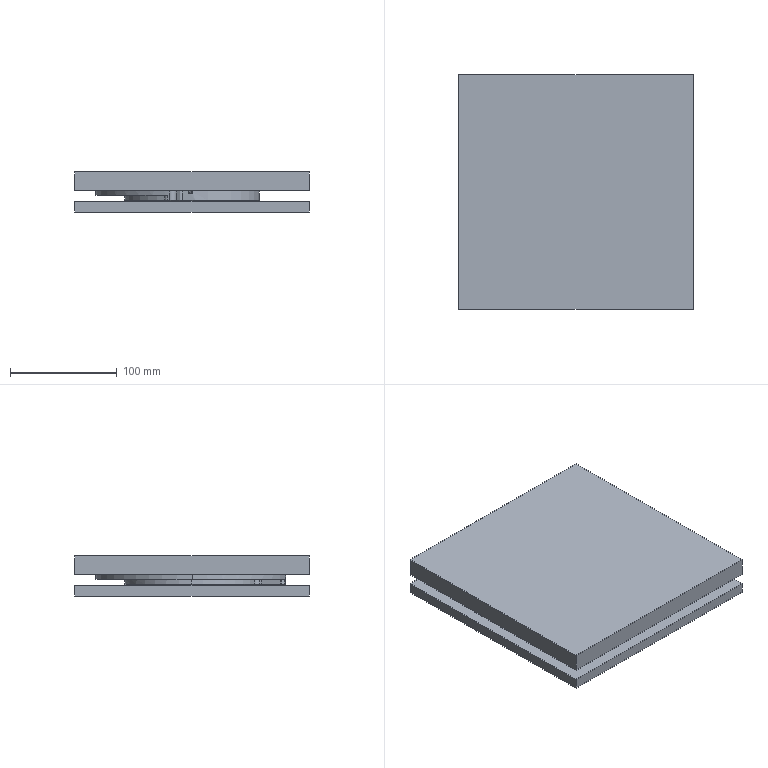NC program | NX | posted with a generic post | part box 220 x 220 x 37.5 mm
Lines 3644 to 4913 of 13716:
(ZLEVEL_PROFILE_COPY , TOOL : D10JING)
N7250 T07 M6
N7252 G54
N7254 G17 G0 G90 X87.471 Y-41.927 S8000 M3
N7256 G43 Z30. H7
N7258 Z-17.
N7260 G94 G1 X85.759 Y-42.028 F1200.
N7262 G3 X84.924 Y-42.578 R1.
N7264 G2 X70.985 Y-46.757 R10.
N7266 G1 X56.243 Y-38.246
N7268 X56.225 Y-38.248
N7270 X55.355 Y-39.494
N7272 G2 X55.057 Y-39.91 R68.
N7274 G1 X54.666 Y-40.443
N7276 G2 X52.455 Y-43.272 R68.
N7278 G1 X52.409 Y-43.328
N7280 G2 X-67.991 Y-1.079 R68.
N7282 G1 X-67.995 Y0.834
N7284 G2 X-67.897 Y3.74 R68.
N7286 G1 X-67.853 Y4.42
N7288 X-67.856 Y4.43
N7290 G2 X-67.657 Y6.818 R68.
N7292 G1 X-67.652 Y6.852
N7294 X-84.432 Y9.81
N7296 G2 X-92.427 Y21.958 R10.
N7298 G1 X-92.42 Y21.99
N7300 G3 X-92.706 Y22.949 R1.
N7302 G1 X-93.952 Y24.125
N7304 G0 Z30.
N7306 M5
(ZLEVEL_PROFILE_COPY_1 , TOOL : D6)
N7308 T09 M6
N7310 G54
N7312 G17 G0 G90 X38.681 Y9.135 S9500 M3
N7314 G43 Z30. H9
N7316 Z-0.5
N7318 G94 G1 X37.71 Y9.242 F1000.
N7320 G3 X37.511 Y8.676 R0.6
N7322 G1 X37.527 Y8.601 F1500.
N7324 G2 X37.907 Y6.73 R38.5
N7326 G1 X39.921 Y6.928
N7328 G3 X40.409 Y7.277 R0.6
N7330 G1 X40.838 Y8.223
N7332 G0 X38.681 Y9.135 Z-1.
N7334 G1 X37.71 Y9.242 F1000.
N7336 G3 X37.511 Y8.676 R0.6
N7338 G1 X37.527 Y8.601 F1500.
N7340 G2 X37.907 Y6.73 R38.5
N7342 G1 X39.921 Y6.928
N7344 G3 X40.409 Y7.277 R0.6
N7346 G1 X40.838 Y8.223
N7348 G0 X38.681 Y9.135 Z-1.5
N7350 G1 X37.71 Y9.242 F1000.
N7352 G3 X37.511 Y8.676 R0.6
N7354 G1 X37.527 Y8.601 F1500.
N7356 G2 X37.907 Y6.73 R38.5
N7358 G1 X39.921 Y6.928
N7360 G3 X40.409 Y7.277 R0.6
N7362 G1 X40.838 Y8.223
N7364 G0 X38.681 Y9.135 Z-2.
N7366 G1 X37.71 Y9.242 F1000.
N7368 G3 X37.511 Y8.676 R0.6
N7370 G1 X37.527 Y8.601 F1500.
N7372 G2 X37.907 Y6.73 R38.5
N7374 G1 X39.921 Y6.928
N7376 G3 X40.409 Y7.277 R0.6
N7378 G1 X40.838 Y8.223
N7380 G0 X38.681 Y9.135 Z-2.5
N7382 G1 X37.71 Y9.242 F1000.
N7384 G3 X37.511 Y8.676 R0.6
N7386 G1 X37.527 Y8.601 F1500.
N7388 G2 X37.907 Y6.73 R38.5
N7390 G1 X39.921 Y6.928
N7392 G3 X40.409 Y7.277 R0.6
N7394 G1 X40.838 Y8.223
N7396 G0 X38.681 Y9.135 Z-3.
N7398 G1 X37.71 Y9.242 F1000.
N7400 G3 X37.511 Y8.676 R0.6
N7402 G1 X37.527 Y8.601 F1500.
N7404 G2 X37.907 Y6.73 R38.5
N7406 G1 X39.921 Y6.928
N7408 G3 X40.409 Y7.277 R0.6
N7410 G1 X40.838 Y8.223
N7412 G0 X38.681 Y9.135 Z-3.5
N7414 G1 X37.71 Y9.242 F1000.
N7416 G3 X37.511 Y8.676 R0.6
N7418 G1 X37.527 Y8.601 F1500.
N7420 G2 X37.907 Y6.73 R38.5
N7422 G1 X39.921 Y6.928
N7424 G3 X40.409 Y7.277 R0.6
N7426 G1 X40.838 Y8.223
N7428 G0 X38.681 Y9.135 Z-4.
N7430 G1 X37.71 Y9.242 F1000.
N7432 G3 X37.511 Y8.676 R0.6
N7434 G1 X37.527 Y8.601 F1500.
N7436 G2 X37.907 Y6.73 R38.5
N7438 G1 X39.921 Y6.928
N7440 G3 X40.409 Y7.277 R0.6
N7442 G1 X40.838 Y8.223
N7444 G0 X38.681 Y9.135 Z-4.5
N7446 G1 X37.71 Y9.242 F1000.
N7448 G3 X37.511 Y8.676 R0.6
N7450 G1 X37.527 Y8.601 F1500.
N7452 G2 X37.907 Y6.73 R38.5
N7454 G1 X39.921 Y6.928
N7456 G3 X40.409 Y7.277 R0.6
N7458 G1 X40.838 Y8.223
N7460 G0 X38.681 Y9.135 Z-5.
N7462 G1 X37.71 Y9.242 F1000.
N7464 G3 X37.511 Y8.676 R0.6
N7466 G1 X37.527 Y8.601 F1500.
N7468 G2 X37.907 Y6.73 R38.5
N7470 G1 X39.921 Y6.928
N7472 G3 X40.409 Y7.277 R0.6
N7474 G1 X40.838 Y8.223
N7476 G0 X38.681 Y9.135 Z-5.5
N7478 G1 X37.71 Y9.242 F1000.
N7480 G3 X37.511 Y8.676 R0.6
N7482 G1 X37.527 Y8.601 F1500.
N7484 G2 X37.907 Y6.73 R38.5
N7486 G1 X39.921 Y6.928
N7488 G3 X40.409 Y7.277 R0.6
N7490 G1 X40.838 Y8.223
N7492 G0 X38.681 Y9.135 Z-6.
N7494 G1 X37.71 Y9.242 F1000.
N7496 G3 X37.511 Y8.676 R0.6
N7498 G1 X37.527 Y8.601 F1500.
N7500 G2 X37.907 Y6.73 R38.5
N7502 G1 X39.921 Y6.928
N7504 G3 X40.409 Y7.277 R0.6
N7506 G1 X40.838 Y8.223
N7508 G0 X38.681 Y9.135 Z-6.5
N7510 G1 X37.71 Y9.242 F1000.
N7512 G3 X37.511 Y8.676 R0.6
N7514 G1 X37.527 Y8.601 F1500.
N7516 G2 X37.907 Y6.73 R38.5
N7518 G1 X39.921 Y6.928
N7520 G3 X40.409 Y7.277 R0.6
N7522 G1 X40.838 Y8.223
N7524 G0 X38.681 Y9.135 Z-7.
N7526 G1 X37.71 Y9.242 F1000.
N7528 G3 X37.511 Y8.676 R0.6
N7530 G1 X37.527 Y8.601 F1500.
N7532 G2 X37.907 Y6.73 R38.5
N7534 G1 X39.921 Y6.928
N7536 G3 X40.409 Y7.277 R0.6
N7538 G1 X40.838 Y8.223
N7540 G0 X38.681 Y9.135 Z-7.5
N7542 G1 X37.71 Y9.242 F1000.
N7544 G3 X37.511 Y8.676 R0.6
N7546 G1 X37.527 Y8.601 F1500.
N7548 G2 X37.907 Y6.73 R38.5
N7550 G1 X39.921 Y6.928
N7552 G3 X40.409 Y7.277 R0.6
N7554 G1 X40.838 Y8.223
N7556 G0 X38.681 Y9.135 Z-8.
N7558 G1 X37.71 Y9.242 F1000.
N7560 G3 X37.511 Y8.676 R0.6
N7562 G1 X37.527 Y8.601 F1500.
N7564 G2 X37.907 Y6.73 R38.5
N7566 G1 X39.921 Y6.928
N7568 G3 X40.409 Y7.277 R0.6
N7570 G1 X40.838 Y8.223
N7572 G0 X38.681 Y9.135 Z-8.5
N7574 G1 X37.71 Y9.242 F1000.
N7576 G3 X37.511 Y8.676 R0.6
N7578 G1 X37.527 Y8.601 F1500.
N7580 G2 X37.907 Y6.73 R38.5
N7582 G1 X39.921 Y6.928
N7584 G3 X40.409 Y7.277 R0.6
N7586 G1 X40.838 Y8.223
N7588 G0 X38.681 Y9.135 Z-9.
N7590 G1 X37.71 Y9.242 F1000.
N7592 G3 X37.511 Y8.676 R0.6
N7594 G1 X37.527 Y8.601 F1500.
N7596 G2 X37.907 Y6.73 R38.5
N7598 G1 X39.921 Y6.928
N7600 G3 X40.409 Y7.277 R0.6
N7602 G1 X40.838 Y8.223
N7604 G0 X38.681 Y9.135 Z-9.5
N7606 G1 X37.71 Y9.242 F1000.
N7608 G3 X37.511 Y8.676 R0.6
N7610 G1 X37.527 Y8.601 F1500.
N7612 G2 X37.907 Y6.73 R38.5
N7614 G1 X39.921 Y6.928
N7616 G3 X40.409 Y7.277 R0.6
N7618 G1 X40.838 Y8.223
N7620 G0 X38.681 Y9.135 Z-10.
N7622 G1 X37.71 Y9.242 F1000.
N7624 G3 X37.511 Y8.676 R0.6
N7626 G1 X37.527 Y8.601 F1500.
N7628 G2 X37.907 Y6.73 R38.5
N7630 G1 X39.921 Y6.928
N7632 G3 X40.409 Y7.277 R0.6
N7634 G1 X40.838 Y8.223
N7636 G0 Z30.
N7638 X39.099 Y-14.376
N7640 Z-0.5
N7642 G1 X38.819 Y-13.375 F1000.
N7644 G3 X38.391 Y-12.955 R0.6
N7646 G1 X36.431 Y-12.452 F1500.
N7648 G2 X35.74 Y-14.314 R38.5
N7650 G3 X35.826 Y-14.908 R0.6
N7652 G1 X36.458 Y-15.712
N7654 G0 X39.099 Y-14.376 Z-1.
N7656 G1 X38.819 Y-13.375 F1000.
N7658 G3 X38.391 Y-12.955 R0.6
N7660 G1 X36.431 Y-12.452 F1500.
N7662 G2 X35.74 Y-14.314 R38.5
N7664 G3 X35.826 Y-14.908 R0.6
N7666 G1 X36.458 Y-15.712
N7668 G0 X39.099 Y-14.376 Z-1.5
N7670 G1 X38.819 Y-13.375 F1000.
N7672 G3 X38.391 Y-12.955 R0.6
N7674 G1 X36.431 Y-12.452 F1500.
N7676 G2 X35.74 Y-14.314 R38.5
N7678 G3 X35.826 Y-14.908 R0.6
N7680 G1 X36.458 Y-15.712
N7682 G0 X39.099 Y-14.376 Z-2.
N7684 G1 X38.819 Y-13.375 F1000.
N7686 G3 X38.391 Y-12.955 R0.6
N7688 G1 X36.431 Y-12.452 F1500.
N7690 G2 X35.74 Y-14.314 R38.5
N7692 G3 X35.826 Y-14.908 R0.6
N7694 G1 X36.458 Y-15.712
N7696 G0 X39.099 Y-14.376 Z-2.5
N7698 G1 X38.819 Y-13.375 F1000.
N7700 G3 X38.391 Y-12.955 R0.6
N7702 G1 X36.431 Y-12.452 F1500.
N7704 G2 X35.74 Y-14.314 R38.5
N7706 G3 X35.826 Y-14.908 R0.6
N7708 G1 X36.458 Y-15.712
N7710 G0 X39.099 Y-14.376 Z-3.
N7712 G1 X38.819 Y-13.375 F1000.
N7714 G3 X38.391 Y-12.955 R0.6
N7716 G1 X36.431 Y-12.452 F1500.
N7718 G2 X35.74 Y-14.314 R38.5
N7720 G3 X35.826 Y-14.908 R0.6
N7722 G1 X36.458 Y-15.712
N7724 G0 X39.099 Y-14.376 Z-3.5
N7726 G1 X38.819 Y-13.375 F1000.
N7728 G3 X38.391 Y-12.955 R0.6
N7730 G1 X36.431 Y-12.452 F1500.
N7732 G2 X35.74 Y-14.314 R38.5
N7734 G3 X35.826 Y-14.908 R0.6
N7736 G1 X36.458 Y-15.712
N7738 G0 X39.099 Y-14.376 Z-4.
N7740 G1 X38.819 Y-13.375 F1000.
N7742 G3 X38.391 Y-12.955 R0.6
N7744 G1 X36.431 Y-12.452 F1500.
N7746 G2 X35.74 Y-14.314 R38.5
N7748 G3 X35.826 Y-14.908 R0.6
N7750 G1 X36.458 Y-15.712
N7752 G0 X39.099 Y-14.376 Z-4.5
N7754 G1 X38.819 Y-13.375 F1000.
N7756 G3 X38.391 Y-12.955 R0.6
N7758 G1 X36.431 Y-12.452 F1500.
N7760 G2 X35.74 Y-14.314 R38.5
N7762 G3 X35.826 Y-14.908 R0.6
N7764 G1 X36.458 Y-15.712
N7766 G0 X39.099 Y-14.376 Z-5.
N7768 G1 X38.819 Y-13.375 F1000.
N7770 G3 X38.391 Y-12.955 R0.6
N7772 G1 X36.431 Y-12.452 F1500.
N7774 G2 X35.74 Y-14.314 R38.5
N7776 G3 X35.826 Y-14.908 R0.6
N7778 G1 X36.458 Y-15.712
N7780 G0 X39.099 Y-14.376 Z-5.5
N7782 G1 X38.819 Y-13.375 F1000.
N7784 G3 X38.391 Y-12.955 R0.6
N7786 G1 X36.431 Y-12.452 F1500.
N7788 G2 X35.74 Y-14.314 R38.5
N7790 G3 X35.826 Y-14.908 R0.6
N7792 G1 X36.458 Y-15.712
N7794 G0 X39.099 Y-14.376 Z-6.
N7796 G1 X38.819 Y-13.375 F1000.
N7798 G3 X38.391 Y-12.955 R0.6
N7800 G1 X36.431 Y-12.452 F1500.
N7802 G2 X35.74 Y-14.314 R38.5
N7804 G3 X35.826 Y-14.908 R0.6
N7806 G1 X36.458 Y-15.712
N7808 G0 X39.099 Y-14.376 Z-6.5
N7810 G1 X38.819 Y-13.375 F1000.
N7812 G3 X38.391 Y-12.955 R0.6
N7814 G1 X36.431 Y-12.452 F1500.
N7816 G2 X35.74 Y-14.314 R38.5
N7818 G3 X35.826 Y-14.908 R0.6
N7820 G1 X36.458 Y-15.712
N7822 G0 X39.099 Y-14.376 Z-7.
N7824 G1 X38.819 Y-13.375 F1000.
N7826 G3 X38.391 Y-12.955 R0.6
N7828 G1 X36.431 Y-12.452 F1500.
N7830 G2 X35.74 Y-14.314 R38.5
N7832 G3 X35.826 Y-14.908 R0.6
N7834 G1 X36.458 Y-15.712
N7836 G0 X39.099 Y-14.376 Z-7.5
N7838 G1 X38.819 Y-13.375 F1000.
N7840 G3 X38.391 Y-12.955 R0.6
N7842 G1 X36.431 Y-12.452 F1500.
N7844 G2 X35.74 Y-14.314 R38.5
N7846 G3 X35.826 Y-14.908 R0.6
N7848 G1 X36.458 Y-15.712
N7850 G0 X39.099 Y-14.376 Z-8.
N7852 G1 X38.819 Y-13.375 F1000.
N7854 G3 X38.391 Y-12.955 R0.6
N7856 G1 X36.431 Y-12.452 F1500.
N7858 G2 X35.74 Y-14.314 R38.5
N7860 G3 X35.826 Y-14.908 R0.6
N7862 G1 X36.458 Y-15.712
N7864 G0 X39.099 Y-14.376 Z-8.5
N7866 G1 X38.819 Y-13.375 F1000.
N7868 G3 X38.391 Y-12.955 R0.6
N7870 G1 X36.431 Y-12.452 F1500.
N7872 G2 X35.74 Y-14.314 R38.5
N7874 G3 X35.826 Y-14.908 R0.6
N7876 G1 X36.458 Y-15.712
N7878 G0 X39.099 Y-14.376 Z-9.
N7880 G1 X38.819 Y-13.375 F1000.
N7882 G3 X38.391 Y-12.955 R0.6
N7884 G1 X36.431 Y-12.452 F1500.
N7886 G2 X35.74 Y-14.314 R38.5
N7888 G3 X35.826 Y-14.908 R0.6
N7890 G1 X36.458 Y-15.712
N7892 G0 X39.099 Y-14.376 Z-9.5
N7894 G1 X38.819 Y-13.375 F1000.
N7896 G3 X38.391 Y-12.955 R0.6
N7898 G1 X36.431 Y-12.452 F1500.
N7900 G2 X35.74 Y-14.314 R38.5
N7902 G3 X35.826 Y-14.908 R0.6
N7904 G1 X36.458 Y-15.712
N7906 G0 X39.099 Y-14.376 Z-10.
N7908 G1 X38.819 Y-13.375 F1000.
N7910 G3 X38.391 Y-12.955 R0.6
N7912 G1 X36.431 Y-12.452 F1500.
N7914 G2 X35.74 Y-14.314 R38.5
N7916 G3 X35.826 Y-14.908 R0.6
N7918 G1 X36.458 Y-15.712
N7920 G0 Z30.
N7922 X-33.176 Y-21.805
N7924 Z-0.5
N7926 G1 X-32.693 Y-20.902 F1000.
N7928 G3 X-32.712 Y-20.302 R0.6
N7930 G2 X-33.715 Y-18.589 R38.5 F1500.
N7932 G1 X-35.558 Y-19.425
N7934 G3 X-35.907 Y-19.913 R0.6
N7936 G1 X-36.009 Y-20.947
N7938 G0 X-33.176 Y-21.805 Z-1.
N7940 G1 X-32.693 Y-20.902 F1000.
N7942 G3 X-32.712 Y-20.302 R0.6
N7944 G2 X-33.715 Y-18.589 R38.5 F1500.
N7946 G1 X-35.558 Y-19.425
N7948 G3 X-35.907 Y-19.913 R0.6
N7950 G1 X-36.009 Y-20.947
N7952 G0 X-33.176 Y-21.805 Z-1.5
N7954 G1 X-32.693 Y-20.902 F1000.
N7956 G3 X-32.712 Y-20.302 R0.6
N7958 G2 X-33.715 Y-18.589 R38.5 F1500.
N7960 G1 X-35.558 Y-19.425
N7962 G3 X-35.907 Y-19.913 R0.6
N7964 G1 X-36.009 Y-20.947
N7966 G0 X-33.176 Y-21.805 Z-2.
N7968 G1 X-32.693 Y-20.902 F1000.
N7970 G3 X-32.712 Y-20.302 R0.6
N7972 G2 X-33.715 Y-18.589 R38.5 F1500.
N7974 G1 X-35.558 Y-19.425
N7976 G3 X-35.907 Y-19.913 R0.6
N7978 G1 X-36.009 Y-20.947
N7980 G0 X-33.176 Y-21.805 Z-2.5
N7982 G1 X-32.693 Y-20.902 F1000.
N7984 G3 X-32.712 Y-20.302 R0.6
N7986 G2 X-33.715 Y-18.589 R38.5 F1500.
N7988 G1 X-35.558 Y-19.425
N7990 G3 X-35.907 Y-19.913 R0.6
N7992 G1 X-36.009 Y-20.947
N7994 G0 X-33.176 Y-21.805 Z-3.
N7996 G1 X-32.693 Y-20.902 F1000.
N7998 G3 X-32.712 Y-20.302 R0.6
N8000 G2 X-33.715 Y-18.589 R38.5 F1500.
N8002 G1 X-35.558 Y-19.425
N8004 G3 X-35.907 Y-19.913 R0.6
N8006 G1 X-36.009 Y-20.947
N8008 G0 X-33.176 Y-21.805 Z-3.5
N8010 G1 X-32.693 Y-20.902 F1000.
N8012 G3 X-32.712 Y-20.302 R0.6
N8014 G2 X-33.715 Y-18.589 R38.5 F1500.
N8016 G1 X-35.558 Y-19.425
N8018 G3 X-35.907 Y-19.913 R0.6
N8020 G1 X-36.009 Y-20.947
N8022 G0 X-33.176 Y-21.805 Z-4.
N8024 G1 X-32.693 Y-20.902 F1000.
N8026 G3 X-32.712 Y-20.302 R0.6
N8028 G2 X-33.715 Y-18.589 R38.5 F1500.
N8030 G1 X-35.558 Y-19.425
N8032 G3 X-35.907 Y-19.913 R0.6
N8034 G1 X-36.009 Y-20.947
N8036 G0 X-33.176 Y-21.805 Z-4.5
N8038 G1 X-32.693 Y-20.902 F1000.
N8040 G3 X-32.712 Y-20.302 R0.6
N8042 G2 X-33.715 Y-18.589 R38.5 F1500.
N8044 G1 X-35.558 Y-19.425
N8046 G3 X-35.907 Y-19.913 R0.6
N8048 G1 X-36.009 Y-20.947
N8050 G0 X-33.176 Y-21.805 Z-5.
N8052 G1 X-32.693 Y-20.902 F1000.
N8054 G3 X-32.712 Y-20.302 R0.6
N8056 G2 X-33.715 Y-18.589 R38.5 F1500.
N8058 G1 X-35.558 Y-19.425
N8060 G3 X-35.907 Y-19.913 R0.6
N8062 G1 X-36.009 Y-20.947
N8064 G0 X-33.176 Y-21.805 Z-5.5
N8066 G1 X-32.693 Y-20.902 F1000.
N8068 G3 X-32.712 Y-20.302 R0.6
N8070 G2 X-33.715 Y-18.589 R38.5 F1500.
N8072 G1 X-35.558 Y-19.425
N8074 G3 X-35.907 Y-19.913 R0.6
N8076 G1 X-36.009 Y-20.947
N8078 G0 X-33.176 Y-21.805 Z-6.
N8080 G1 X-32.693 Y-20.902 F1000.
N8082 G3 X-32.712 Y-20.302 R0.6
N8084 G2 X-33.715 Y-18.589 R38.5 F1500.
N8086 G1 X-35.558 Y-19.425
N8088 G3 X-35.907 Y-19.913 R0.6
N8090 G1 X-36.009 Y-20.947
N8092 G0 X-33.176 Y-21.805 Z-6.5
N8094 G1 X-32.693 Y-20.902 F1000.
N8096 G3 X-32.712 Y-20.302 R0.6
N8098 G2 X-33.715 Y-18.589 R38.5 F1500.
N8100 G1 X-35.558 Y-19.425
N8102 G3 X-35.907 Y-19.913 R0.6
N8104 G1 X-36.009 Y-20.947
N8106 G0 X-33.176 Y-21.805 Z-7.
N8108 G1 X-32.693 Y-20.902 F1000.
N8110 G3 X-32.712 Y-20.302 R0.6
N8112 G2 X-33.715 Y-18.589 R38.5 F1500.
N8114 G1 X-35.558 Y-19.425
N8116 G3 X-35.907 Y-19.913 R0.6
N8118 G1 X-36.009 Y-20.947
N8120 G0 X-33.176 Y-21.805 Z-7.5
N8122 G1 X-32.693 Y-20.902 F1000.
N8124 G3 X-32.712 Y-20.302 R0.6
N8126 G2 X-33.715 Y-18.589 R38.5 F1500.
N8128 G1 X-35.558 Y-19.425
N8130 G3 X-35.907 Y-19.913 R0.6
N8132 G1 X-36.009 Y-20.947
N8134 G0 X-33.176 Y-21.805 Z-8.
N8136 G1 X-32.693 Y-20.902 F1000.
N8138 G3 X-32.712 Y-20.302 R0.6
N8140 G2 X-33.715 Y-18.589 R38.5 F1500.
N8142 G1 X-35.558 Y-19.425
N8144 G3 X-35.907 Y-19.913 R0.6
N8146 G1 X-36.009 Y-20.947
N8148 G0 X-33.176 Y-21.805 Z-8.5
N8150 G1 X-32.693 Y-20.902 F1000.
N8152 G3 X-32.712 Y-20.302 R0.6
N8154 G2 X-33.715 Y-18.589 R38.5 F1500.
N8156 G1 X-35.558 Y-19.425
N8158 G3 X-35.907 Y-19.913 R0.6
N8160 G1 X-36.009 Y-20.947
N8162 G0 X-33.176 Y-21.805 Z-9.
N8164 G1 X-32.693 Y-20.902 F1000.
N8166 G3 X-32.712 Y-20.302 R0.6
N8168 G2 X-33.715 Y-18.589 R38.5 F1500.
N8170 G1 X-35.558 Y-19.425
N8172 G3 X-35.907 Y-19.913 R0.6
N8174 G1 X-36.009 Y-20.947
N8176 G0 X-33.176 Y-21.805 Z-9.5
N8178 G1 X-32.693 Y-20.902 F1000.
N8180 G3 X-32.712 Y-20.302 R0.6
N8182 G2 X-33.715 Y-18.589 R38.5 F1500.
N8184 G1 X-35.558 Y-19.425
N8186 G3 X-35.907 Y-19.913 R0.6
N8188 G1 X-36.009 Y-20.947
N8190 G0 X-33.176 Y-21.805 Z-10.
N8192 G1 X-32.693 Y-20.902 F1000.
N8194 G3 X-32.712 Y-20.302 R0.6
N8196 G2 X-33.715 Y-18.589 R38.5 F1500.
N8198 G1 X-35.558 Y-19.425
N8200 G3 X-35.907 Y-19.913 R0.6
N8202 G1 X-36.009 Y-20.947
N8204 G0 Z30.
N8206 X-41.4 Y4.633
N8208 Z-0.5
N8210 G1 X-40.89 Y3.727 F1000.
N8212 G3 X-40.373 Y3.422 R0.6
N8214 G1 X-38.349 Y3.401 F1500.
N8216 G2 X-38.123 Y5.374 R38.5
N8218 G3 X-38.348 Y5.93 R0.6
N8220 G1 X-39.154 Y6.561
N8222 G0 X-41.4 Y4.633 Z-1.
N8224 G1 X-40.89 Y3.727 F1000.
N8226 G3 X-40.373 Y3.422 R0.6
N8228 G1 X-38.349 Y3.401 F1500.
N8230 G2 X-38.123 Y5.374 R38.5
N8232 G3 X-38.348 Y5.93 R0.6
N8234 G1 X-39.154 Y6.561
N8236 G0 X-41.4 Y4.633 Z-1.5
N8238 G1 X-40.89 Y3.727 F1000.
N8240 G3 X-40.373 Y3.422 R0.6
N8242 G1 X-38.349 Y3.401 F1500.
N8244 G2 X-38.123 Y5.374 R38.5
N8246 G3 X-38.348 Y5.93 R0.6
N8248 G1 X-39.154 Y6.561
N8250 G0 X-41.4 Y4.633 Z-2.
N8252 G1 X-40.89 Y3.727 F1000.
N8254 G3 X-40.373 Y3.422 R0.6
N8256 G1 X-38.349 Y3.401 F1500.
N8258 G2 X-38.123 Y5.374 R38.5
N8260 G3 X-38.348 Y5.93 R0.6
N8262 G1 X-39.154 Y6.561
N8264 G0 X-41.4 Y4.633 Z-2.5
N8266 G1 X-40.89 Y3.727 F1000.
N8268 G3 X-40.373 Y3.422 R0.6
N8270 G1 X-38.349 Y3.401 F1500.
N8272 G2 X-38.123 Y5.374 R38.5
N8274 G3 X-38.348 Y5.93 R0.6
N8276 G1 X-39.154 Y6.561
N8278 G0 X-41.4 Y4.633 Z-3.
N8280 G1 X-40.89 Y3.727 F1000.
N8282 G3 X-40.373 Y3.422 R0.6
N8284 G1 X-38.349 Y3.401 F1500.
N8286 G2 X-38.123 Y5.374 R38.5
N8288 G3 X-38.348 Y5.93 R0.6
N8290 G1 X-39.154 Y6.561
N8292 G0 X-41.4 Y4.633 Z-3.5
N8294 G1 X-40.89 Y3.727 F1000.
N8296 G3 X-40.373 Y3.422 R0.6
N8298 G1 X-38.349 Y3.401 F1500.
N8300 G2 X-38.123 Y5.374 R38.5
N8302 G3 X-38.348 Y5.93 R0.6
N8304 G1 X-39.154 Y6.561
N8306 G0 X-41.4 Y4.633 Z-4.
N8308 G1 X-40.89 Y3.727 F1000.
N8310 G3 X-40.373 Y3.422 R0.6
N8312 G1 X-38.349 Y3.401 F1500.
N8314 G2 X-38.123 Y5.374 R38.5
N8316 G3 X-38.348 Y5.93 R0.6
N8318 G1 X-39.154 Y6.561
N8320 G0 X-41.4 Y4.633 Z-4.5
N8322 G1 X-40.89 Y3.727 F1000.
N8324 G3 X-40.373 Y3.422 R0.6
N8326 G1 X-38.349 Y3.401 F1500.
N8328 G2 X-38.123 Y5.374 R38.5
N8330 G3 X-38.348 Y5.93 R0.6
N8332 G1 X-39.154 Y6.561
N8334 G0 X-41.4 Y4.633 Z-5.
N8336 G1 X-40.89 Y3.727 F1000.
N8338 G3 X-40.373 Y3.422 R0.6
N8340 G1 X-38.349 Y3.401 F1500.
N8342 G2 X-38.123 Y5.374 R38.5
N8344 G3 X-38.348 Y5.93 R0.6
N8346 G1 X-39.154 Y6.561
N8348 G0 X-41.4 Y4.633 Z-5.5
N8350 G1 X-40.89 Y3.727 F1000.
N8352 G3 X-40.373 Y3.422 R0.6
N8354 G1 X-38.349 Y3.401 F1500.
N8356 G2 X-38.123 Y5.374 R38.5
N8358 G3 X-38.348 Y5.93 R0.6
N8360 G1 X-39.154 Y6.561
N8362 G0 X-41.4 Y4.633 Z-6.
N8364 G1 X-40.89 Y3.727 F1000.
N8366 G3 X-40.373 Y3.422 R0.6
N8368 G1 X-38.349 Y3.401 F1500.
N8370 G2 X-38.123 Y5.374 R38.5
N8372 G3 X-38.348 Y5.93 R0.6
N8374 G1 X-39.154 Y6.561
N8376 G0 X-41.4 Y4.633 Z-6.5
N8378 G1 X-40.89 Y3.727 F1000.
N8380 G3 X-40.373 Y3.422 R0.6
N8382 G1 X-38.349 Y3.401 F1500.
N8384 G2 X-38.123 Y5.374 R38.5
N8386 G3 X-38.348 Y5.93 R0.6
N8388 G1 X-39.154 Y6.561
N8390 G0 X-41.4 Y4.633 Z-7.
N8392 G1 X-40.89 Y3.727 F1000.
N8394 G3 X-40.373 Y3.422 R0.6
N8396 G1 X-38.349 Y3.401 F1500.
N8398 G2 X-38.123 Y5.374 R38.5
N8400 G3 X-38.348 Y5.93 R0.6
N8402 G1 X-39.154 Y6.561
N8404 G0 X-41.4 Y4.633 Z-7.5
N8406 G1 X-40.89 Y3.727 F1000.
N8408 G3 X-40.373 Y3.422 R0.6
N8410 G1 X-38.349 Y3.401 F1500.
N8412 G2 X-38.123 Y5.374 R38.5
N8414 G3 X-38.348 Y5.93 R0.6
N8416 G1 X-39.154 Y6.561
N8418 G0 X-41.4 Y4.633 Z-8.
N8420 G1 X-40.89 Y3.727 F1000.
N8422 G3 X-40.373 Y3.422 R0.6
N8424 G1 X-38.349 Y3.401 F1500.
N8426 G2 X-38.123 Y5.374 R38.5
N8428 G3 X-38.348 Y5.93 R0.6
N8430 G1 X-39.154 Y6.561
N8432 G0 X-41.4 Y4.633 Z-8.5
N8434 G1 X-40.89 Y3.727 F1000.
N8436 G3 X-40.373 Y3.422 R0.6
N8438 G1 X-38.349 Y3.401 F1500.
N8440 G2 X-38.123 Y5.374 R38.5
N8442 G3 X-38.348 Y5.93 R0.6
N8444 G1 X-39.154 Y6.561
N8446 G0 X-41.4 Y4.633 Z-9.
N8448 G1 X-40.89 Y3.727 F1000.
N8450 G3 X-40.373 Y3.422 R0.6
N8452 G1 X-38.349 Y3.401 F1500.
N8454 G2 X-38.123 Y5.374 R38.5
N8456 G3 X-38.348 Y5.93 R0.6
N8458 G1 X-39.154 Y6.561
N8460 G0 X-41.4 Y4.633 Z-9.5
N8462 G1 X-40.89 Y3.727 F1000.
N8464 G3 X-40.373 Y3.422 R0.6
N8466 G1 X-38.349 Y3.401 F1500.
N8468 G2 X-38.123 Y5.374 R38.5
N8470 G3 X-38.348 Y5.93 R0.6
N8472 G1 X-39.154 Y6.561
N8474 G0 X-41.4 Y4.633 Z-10.
N8476 G1 X-40.89 Y3.727 F1000.
N8478 G3 X-40.373 Y3.422 R0.6
N8480 G1 X-38.349 Y3.401 F1500.
N8482 G2 X-38.123 Y5.374 R38.5
N8484 G3 X-38.348 Y5.93 R0.6
N8486 G1 X-39.154 Y6.561
N8488 G0 Z30.
N8490 X57.701 Y-38.163
N8492 Z-0.5
N8494 G1 Y-37.124 F1000.
N8496 G3 X57.401 Y-36.604 R0.6
N8498 G1 X55.599 Y-35.564 F1500.
N8500 G2 X54.456 Y-37.289 R66.
N8502 G3 X54.41 Y-37.888 R0.6
N8504 G1 X54.855 Y-38.817
N8506 G0 X57.701 Y-38.163 Z-1.
N8508 G1 Y-37.124 F1000.
N8510 G3 X57.401 Y-36.605 R0.6
N8512 G1 X55.599 Y-35.564 F1500.
N8514 G2 X54.456 Y-37.29 R66.
N8516 G3 X54.41 Y-37.888 R0.6
N8518 G1 X54.855 Y-38.817
N8520 G0 X57.701 Y-38.164 Z-1.5
N8522 G1 Y-37.124 F1000.
N8524 G3 X57.401 Y-36.605 R0.6
N8526 G1 X55.599 Y-35.564 F1500.
N8528 G2 X54.456 Y-37.29 R66.
N8530 G3 X54.41 Y-37.888 R0.6
N8532 G1 X54.855 Y-38.817
N8534 G0 X57.702 Y-38.164 Z-2.
N8536 G1 Y-37.125 F1000.
N8538 G3 X57.402 Y-36.605 R0.6
N8540 G1 X55.599 Y-35.564 F1500.
N8542 G2 X54.456 Y-37.29 R66.
N8544 G3 X54.41 Y-37.889 R0.6
N8546 G1 X54.855 Y-38.818
N8548 G0 X57.702 Y-38.164 Z-2.5
N8550 G1 Y-37.125 F1000.
N8552 G3 X57.402 Y-36.605 R0.6
N8554 G1 X55.599 Y-35.564 F1500.
N8556 G2 X54.456 Y-37.291 R66.
N8558 G3 X54.409 Y-37.889 R0.6
N8560 G1 X54.854 Y-38.818
N8562 G0 X57.702 Y-38.164 Z-3.
N8564 G1 Y-37.125 F1000.
N8566 G3 X57.402 Y-36.605 R0.6
N8568 G1 X55.599 Y-35.564 F1500.
N8570 G2 X54.455 Y-37.291 R66.
N8572 G3 X54.409 Y-37.889 R0.6
N8574 G1 X54.854 Y-38.818
N8576 G0 X57.703 Y-38.164 Z-3.5
N8578 G1 Y-37.125 F1000.
N8580 G3 X57.403 Y-36.606 R0.6
N8582 G1 X55.599 Y-35.564 F1500.
N8584 G2 X54.455 Y-37.291 R66.
N8586 G3 X54.409 Y-37.89 R0.6
N8588 G1 X54.854 Y-38.819
N8590 G0 X57.703 Y-38.165 Z-4.
N8592 G1 Y-37.125 F1000.
N8594 G3 X57.403 Y-36.606 R0.6
N8596 G1 X55.599 Y-35.564 F1500.
N8598 G2 X54.455 Y-37.292 R66.
N8600 G3 X54.409 Y-37.89 R0.6
N8602 G1 X54.854 Y-38.819
N8604 G0 X57.703 Y-38.165 Z-4.5
N8606 G1 Y-37.126 F1000.
N8608 G3 X57.403 Y-36.606 R0.6
N8610 G1 X55.599 Y-35.564 F1500.
N8612 G2 X54.455 Y-37.292 R66.
N8614 G3 X54.409 Y-37.89 R0.6
N8616 G1 X54.854 Y-38.819
N8618 G0 X57.704 Y-38.165 Z-5.
N8620 G1 Y-37.126 F1000.
N8622 G3 X57.404 Y-36.606 R0.6
N8624 G1 X55.599 Y-35.564 F1500.
N8626 G2 X54.454 Y-37.292 R66.
N8628 G3 X54.408 Y-37.891 R0.6
N8630 G1 X54.853 Y-38.82
N8632 G0 X57.704 Y-38.165 Z-5.5
N8634 G1 Y-37.126 F1000.
N8636 G3 X57.404 Y-36.606 R0.6
N8638 G1 X55.599 Y-35.564 F1500.
N8640 G2 X54.454 Y-37.293 R66.
N8642 G3 X54.408 Y-37.891 R0.6
N8644 G1 X54.853 Y-38.82
N8646 G0 X57.704 Y-38.165 Z-6.
N8648 G1 Y-37.126 F1000.
N8650 G3 X57.404 Y-36.606 R0.6
N8652 G1 X55.599 Y-35.564 F1500.
N8654 G2 X54.454 Y-37.293 R66.
N8656 G3 X54.408 Y-37.891 R0.6
N8658 G1 X54.853 Y-38.82
N8660 G0 X57.705 Y-38.166 Z-6.5
N8662 G1 Y-37.126 F1000.
N8664 G3 X57.405 Y-36.607 R0.6
N8666 G1 X55.599 Y-35.564 F1500.
N8668 G2 X54.454 Y-37.293 R66.
N8670 G3 X54.408 Y-37.892 R0.6
N8672 G1 X54.853 Y-38.82
N8674 G0 X57.705 Y-38.166 Z-7.
N8676 G1 Y-37.127 F1000.
N8678 G3 X57.405 Y-36.607 R0.6
N8680 G1 X55.599 Y-35.564 F1500.
N8682 G2 X54.453 Y-37.294 R66.
N8684 G3 X54.407 Y-37.892 R0.6
N8686 G1 X54.852 Y-38.821
N8688 G0 X57.705 Y-38.166 Z-7.5
N8690 G1 Y-37.127 F1000.
N8692 G3 X57.405 Y-36.607 R0.6
N8694 G1 X55.599 Y-35.564 F1500.
N8696 G2 X54.453 Y-37.294 R66.
N8698 G3 X54.407 Y-37.892 R0.6
N8700 G1 X54.852 Y-38.821
N8702 G0 X57.706 Y-38.166 Z-8.
N8704 G1 Y-37.127 F1000.
N8706 G3 X57.406 Y-36.607 R0.6
N8708 G1 X55.599 Y-35.564 F1500.
N8710 G2 X54.453 Y-37.294 R66.
N8712 G3 X54.407 Y-37.892 R0.6
N8714 G1 X54.852 Y-38.821
N8716 G0 X57.706 Y-38.166 Z-8.5
N8718 G1 Y-37.127 F1000.
N8720 G3 X57.406 Y-36.608 R0.6
N8722 G1 X55.599 Y-35.564 F1500.
N8724 G2 X54.453 Y-37.294 R66.
N8726 G3 X54.407 Y-37.892 R0.6
N8728 G1 X54.852 Y-38.821
N8730 G0 X57.707 Y-38.167 Z-9.
N8732 G1 Y-37.128 F1000.
N8734 G3 X57.407 Y-36.608 R0.6
N8736 G1 X55.599 Y-35.564 F1500.
N8738 G2 X54.453 Y-37.294 R66.
N8740 G3 X54.407 Y-37.892 R0.6
N8742 G1 X54.852 Y-38.821
N8744 G0 X57.708 Y-38.167 Z-9.5
N8746 G1 Y-37.128 F1000.
N8748 G3 X57.408 Y-36.608 R0.6
N8750 G1 X55.599 Y-35.564 F1500.
N8752 G2 X54.453 Y-37.294 R66.
N8754 G3 X54.407 Y-37.893 R0.6
N8756 G1 X54.852 Y-38.822
N8758 G0 X57.708 Y-38.168 Z-10.
N8760 G1 Y-37.128 F1000.
N8762 G3 X57.408 Y-36.609 R0.6
N8764 G1 X55.599 Y-35.564 F1500.
N8766 G2 X54.453 Y-37.294 R66.
N8768 G3 X54.407 Y-37.893 R0.6
N8770 G1 X54.852 Y-38.822
N8772 G0 X57.707 Y-38.167 Z-10.5
N8774 G1 Y-37.128 F1000.
N8776 G3 X57.407 Y-36.608 R0.6
N8778 G1 X55.599 Y-35.564 F1500.
N8780 G2 X54.453 Y-37.294 R66.
N8782 G3 X54.407 Y-37.892 R0.6
N8784 G1 X54.852 Y-38.821
N8786 G0 X57.707 Y-38.167 Z-11.
N8788 G1 Y-37.128 F1000.
N8790 G3 X57.407 Y-36.608 R0.6
N8792 G1 X55.599 Y-35.564 F1500.
N8794 G2 X54.453 Y-37.294 R66.
N8796 G3 X54.407 Y-37.892 R0.6
N8798 G1 X54.852 Y-38.821
N8800 G0 X57.707 Y-38.167 Z-11.5
N8802 G1 Y-37.128 F1000.
N8804 G3 X57.407 Y-36.608 R0.6
N8806 G1 X55.599 Y-35.564 F1500.
N8808 G2 X54.453 Y-37.294 R66.
N8810 G3 X54.407 Y-37.893 R0.6
N8812 G1 X54.852 Y-38.821
N8814 G0 X57.708 Y-38.167 Z-12.
N8816 G1 Y-37.128 F1000.
N8818 G3 X57.408 Y-36.608 R0.6
N8820 G1 X55.599 Y-35.564 F1500.
N8822 G2 X54.453 Y-37.294 R66.
N8824 G3 X54.407 Y-37.893 R0.6
N8826 G1 X54.852 Y-38.822
N8828 G0 X55.942 Y-37.234 Z-12.5
N8830 G1 X55.938 Y-36.104 F1000.
N8832 G3 X55.636 Y-35.585 R0.6
N8834 G1 X55.599 Y-35.564 F1500.
N8836 G2 X54.453 Y-37.294 R66.
N8838 G3 X54.407 Y-37.893 R0.6
N8840 G1 X54.852 Y-38.822
N8842 G0 X55.945 Y-37.228 Z-13.
N8844 G1 X55.937 Y-36.101 F1000.
N8846 G3 X55.634 Y-35.584 R0.6
N8848 G1 X55.599 Y-35.564 F1500.
N8850 G2 X54.453 Y-37.294 R66.
N8852 G3 X54.407 Y-37.893 R0.6
N8854 G1 X54.852 Y-38.822
N8856 G0 X55.931 Y-37.25 Z-13.5
N8858 G1 Y-36.102 F1000.
N8860 G3 X55.631 Y-35.583 R0.6
N8862 G1 X55.599 Y-35.564 F1500.
N8864 G2 X54.453 Y-37.294 R66.
N8866 G3 X54.407 Y-37.893 R0.6
N8868 G1 X54.852 Y-38.822
N8870 G0 X55.929 Y-37.254 Z-14.
N8872 G1 Y-36.101 F1000.
N8874 G3 X55.629 Y-35.581 R0.6
N8876 G1 X55.599 Y-35.564 F1500.
N8878 G2 X54.453 Y-37.294 R66.
N8880 G3 X54.407 Y-37.893 R0.6
N8882 G1 X54.852 Y-38.822
N8884 G0 X55.926 Y-37.257 Z-14.5
N8886 G1 Y-36.099 F1000.
N8888 G3 X55.626 Y-35.58 R0.6
N8890 G1 X55.599 Y-35.564 F1500.
N8892 G2 X54.453 Y-37.295 R66.
N8894 G3 X54.407 Y-37.893 R0.6
N8896 G1 X54.852 Y-38.822
N8898 G0 X55.924 Y-37.261 Z-15.
N8900 G1 Y-36.098 F1000.
N8902 G3 X55.624 Y-35.578 R0.6
N8904 G1 X55.599 Y-35.564 F1500.
N8906 G2 X54.453 Y-37.295 R66.
N8908 G3 X54.407 Y-37.893 R0.6
N8910 G1 X54.852 Y-38.822
N8912 G0 X55.921 Y-37.265 Z-15.5
N8914 G1 Y-36.097 F1000.
N8916 G3 X55.621 Y-35.577 R0.6
N8918 G1 X55.599 Y-35.564 F1500.
N8920 G2 X54.453 Y-37.295 R66.
N8922 G3 X54.407 Y-37.893 R0.6
N8924 G1 X54.852 Y-38.822
N8926 G0 X55.919 Y-37.268 Z-16.
N8928 G1 Y-36.095 F1000.
N8930 G3 X55.619 Y-35.576 R0.6
N8932 G1 X55.599 Y-35.564 F1500.
N8934 G2 X54.45 Y-37.299 R66.
N8936 G3 X54.403 Y-37.898 R0.6
N8938 G1 X54.848 Y-38.827
N8940 G0 X55.916 Y-37.272 Z-16.5
N8942 G1 Y-36.094 F1000.
N8944 G3 X55.616 Y-35.574 R0.6
N8946 G1 X55.599 Y-35.564 F1500.
N8948 G2 X54.453 Y-37.295 R66.
N8950 G3 X54.407 Y-37.893 R0.6
N8952 G1 X54.852 Y-38.822
N8954 G0 Z30.
N8956 X-66.973 Y5.517
N8958 Z-0.5
N8960 G1 X-66.035 Y5.943 F1000.
N8962 G3 X-65.686 Y6.431 R0.6
N8964 G2 X-65.451 Y8.495 R66. F1500.
N8966 G1 X-67.52 Y8.859
N8968 G3 X-68.084 Y8.654 R0.6
N8970 G1 X-68.752 Y7.858
N8972 G0 X-66.973 Y5.517 Z-1.
N8974 G1 X-66.035 Y5.943 F1000.
N8976 G3 X-65.686 Y6.431 R0.6
N8978 G2 X-65.451 Y8.495 R66. F1500.
N8980 G1 X-67.52 Y8.859
N8982 G3 X-68.084 Y8.654 R0.6
N8984 G1 X-68.752 Y7.858
N8986 G0 X-66.973 Y5.517 Z-1.5
N8988 G1 X-66.035 Y5.943 F1000.
N8990 G3 X-65.686 Y6.431 R0.6
N8992 G2 X-65.451 Y8.495 R66. F1500.
N8994 G1 X-67.52 Y8.859
N8996 G3 X-68.084 Y8.654 R0.6
N8998 G1 X-68.752 Y7.858
N9000 G0 X-66.973 Y5.517 Z-2.
N9002 G1 X-66.035 Y5.943 F1000.
N9004 G3 X-65.686 Y6.431 R0.6
N9006 G2 X-65.451 Y8.495 R66. F1500.
N9008 G1 X-67.52 Y8.859
N9010 G3 X-68.084 Y8.654 R0.6
N9012 G1 X-68.752 Y7.858
N9014 G0 X-66.973 Y5.517 Z-2.5
N9016 G1 X-66.035 Y5.943 F1000.
N9018 G3 X-65.686 Y6.431 R0.6
N9020 G2 X-65.451 Y8.495 R66. F1500.
N9022 G1 X-67.52 Y8.859
N9024 G3 X-68.084 Y8.654 R0.6
N9026 G1 X-68.752 Y7.858
N9028 G0 X-66.973 Y5.517 Z-3.
N9030 G1 X-66.035 Y5.943 F1000.
N9032 G3 X-65.686 Y6.431 R0.6
N9034 G2 X-65.451 Y8.495 R66. F1500.
N9036 G1 X-67.52 Y8.859
N9038 G3 X-68.084 Y8.654 R0.6
N9040 G1 X-68.752 Y7.858
N9042 G0 X-66.973 Y5.517 Z-3.5
N9044 G1 X-66.035 Y5.943 F1000.
N9046 G3 X-65.686 Y6.431 R0.6
N9048 G2 X-65.451 Y8.495 R66. F1500.
N9050 G1 X-67.52 Y8.859
N9052 G3 X-68.084 Y8.654 R0.6
N9054 G1 X-68.752 Y7.858
N9056 G0 X-66.973 Y5.517 Z-4.
N9058 G1 X-66.035 Y5.943 F1000.
N9060 G3 X-65.686 Y6.431 R0.6
N9062 G2 X-65.451 Y8.495 R66. F1500.
N9064 G1 X-67.52 Y8.859
N9066 G3 X-68.084 Y8.654 R0.6
N9068 G1 X-68.752 Y7.858
N9070 G0 X-66.973 Y5.517 Z-4.5
N9072 G1 X-66.035 Y5.943 F1000.
N9074 G3 X-65.686 Y6.431 R0.6
N9076 G2 X-65.451 Y8.495 R66. F1500.
N9078 G1 X-67.52 Y8.859
N9080 G3 X-68.084 Y8.654 R0.6
N9082 G1 X-68.752 Y7.858
N9084 G0 X-66.973 Y5.517 Z-5.
N9086 G1 X-66.035 Y5.943 F1000.
N9088 G3 X-65.686 Y6.431 R0.6
N9090 G2 X-65.451 Y8.495 R66. F1500.
N9092 G1 X-67.52 Y8.859
N9094 G3 X-68.084 Y8.654 R0.6
N9096 G1 X-68.752 Y7.858
N9098 G0 X-66.973 Y5.517 Z-5.5
N9100 G1 X-66.035 Y5.943 F1000.
N9102 G3 X-65.686 Y6.431 R0.6
N9104 G2 X-65.451 Y8.495 R66. F1500.
N9106 G1 X-67.52 Y8.859
N9108 G3 X-68.084 Y8.654 R0.6
N9110 G1 X-68.752 Y7.858
N9112 G0 X-66.973 Y5.517 Z-6.
N9114 G1 X-66.035 Y5.943 F1000.
N9116 G3 X-65.686 Y6.431 R0.6
N9118 G2 X-65.451 Y8.495 R66. F1500.
N9120 G1 X-67.52 Y8.859
N9122 G3 X-68.084 Y8.654 R0.6
N9124 G1 X-68.752 Y7.858
N9126 G0 X-66.973 Y5.517 Z-6.5
N9128 G1 X-66.035 Y5.943 F1000.
N9130 G3 X-65.686 Y6.431 R0.6
N9132 G2 X-65.451 Y8.495 R66. F1500.
N9134 G1 X-67.52 Y8.859
N9136 G3 X-68.084 Y8.654 R0.6
N9138 G1 X-68.752 Y7.858
N9140 G0 X-66.973 Y5.517 Z-7.
N9142 G1 X-66.035 Y5.943 F1000.
N9144 G3 X-65.686 Y6.431 R0.6
N9146 G2 X-65.451 Y8.495 R66. F1500.
N9148 G1 X-67.52 Y8.859
N9150 G3 X-68.084 Y8.654 R0.6
N9152 G1 X-68.752 Y7.858
N9154 G0 X-66.973 Y5.517 Z-7.5
N9156 G1 X-66.035 Y5.943 F1000.
N9158 G3 X-65.686 Y6.431 R0.6
N9160 G2 X-65.451 Y8.495 R66. F1500.
N9162 G1 X-67.52 Y8.859
N9164 G3 X-68.084 Y8.654 R0.6
N9166 G1 X-68.752 Y7.858
N9168 G0 X-66.973 Y5.517 Z-8.
N9170 G1 X-66.035 Y5.943 F1000.
N9172 G3 X-65.686 Y6.431 R0.6
N9174 G2 X-65.451 Y8.495 R66. F1500.
N9176 G1 X-67.52 Y8.859
N9178 G3 X-68.084 Y8.654 R0.6
N9180 G1 X-68.752 Y7.858
N9182 G0 X-66.973 Y5.517 Z-8.5
N9184 G1 X-66.035 Y5.943 F1000.
N9186 G3 X-65.686 Y6.431 R0.6
N9188 G2 X-65.451 Y8.495 R66. F1500.
N9190 G1 X-67.52 Y8.859
N9192 G3 X-68.084 Y8.654 R0.6
N9194 G1 X-68.752 Y7.858
N9196 G0 X-66.973 Y5.517 Z-9.
N9198 G1 X-66.035 Y5.943 F1000.
N9200 G3 X-65.686 Y6.431 R0.6
N9202 G2 X-65.451 Y8.495 R66. F1500.
N9204 G1 X-67.52 Y8.859
N9206 G3 X-68.084 Y8.654 R0.6
N9208 G1 X-68.752 Y7.858
N9210 G0 X-66.973 Y5.517 Z-9.5
N9212 G1 X-66.035 Y5.943 F1000.
N9214 G3 X-65.686 Y6.431 R0.6
N9216 G2 X-65.451 Y8.495 R66. F1500.
N9218 G1 X-67.52 Y8.859
N9220 G3 X-68.084 Y8.654 R0.6
N9222 G1 X-68.752 Y7.858
N9224 G0 X-66.973 Y5.517 Z-10.
N9226 G1 X-66.035 Y5.943 F1000.
N9228 G3 X-65.686 Y6.431 R0.6
N9230 G2 X-65.451 Y8.495 R66. F1500.
N9232 G1 X-67.52 Y8.859
N9234 G3 X-68.084 Y8.654 R0.6
N9236 G1 X-68.752 Y7.858
N9238 G0 X-66.973 Y5.517 Z-10.5
N9240 G1 X-66.035 Y5.943 F1000.
N9242 G3 X-65.686 Y6.431 R0.6
N9244 G2 X-65.451 Y8.495 R66. F1500.
N9246 G1 X-67.52 Y8.859
N9248 G3 X-68.084 Y8.654 R0.6
N9250 G1 X-68.752 Y7.858
N9252 G0 X-66.973 Y5.517 Z-11.
N9254 G1 X-66.035 Y5.943 F1000.
N9256 G3 X-65.686 Y6.431 R0.6
N9258 G2 X-65.451 Y8.495 R66. F1500.
N9260 G1 X-67.52 Y8.859
N9262 G3 X-68.084 Y8.654 R0.6
N9264 G1 X-68.752 Y7.858
N9266 G0 X-66.973 Y5.517 Z-11.5
N9268 G1 X-66.035 Y5.943 F1000.
N9270 G3 X-65.686 Y6.431 R0.6
N9272 G2 X-65.451 Y8.495 R66. F1500.
N9274 G1 X-67.52 Y8.859
N9276 G3 X-68.084 Y8.654 R0.6
N9278 G1 X-68.752 Y7.858
N9280 G0 X-66.973 Y5.517 Z-12.
N9282 G1 X-66.035 Y5.943 F1000.
N9284 G3 X-65.686 Y6.431 R0.6
N9286 G2 X-65.451 Y8.495 R66. F1500.
N9288 G1 X-67.52 Y8.859
N9290 G3 X-68.084 Y8.654 R0.6
N9292 G1 X-68.752 Y7.858
N9294 G0 X-66.973 Y5.517 Z-12.5
N9296 G1 X-66.035 Y5.943 F1000.
N9298 G3 X-65.686 Y6.431 R0.6
N9300 G2 X-65.451 Y8.495 R66. F1500.
N9302 G1 X-67.52 Y8.859
N9304 G3 X-68.084 Y8.654 R0.6
N9306 G1 X-68.752 Y7.858
N9308 G0 X-66.973 Y5.517 Z-13.
N9310 G1 X-66.035 Y5.943 F1000.
N9312 G3 X-65.686 Y6.431 R0.6
N9314 G2 X-65.451 Y8.495 R66. F1500.
N9316 G1 X-67.52 Y8.859
N9318 G3 X-68.084 Y8.654 R0.6
N9320 G1 X-68.752 Y7.858
N9322 G0 X-66.973 Y5.517 Z-13.5
N9324 G1 X-66.035 Y5.943 F1000.
N9326 G3 X-65.686 Y6.431 R0.6
N9328 G2 X-65.451 Y8.495 R66. F1500.
N9330 G1 X-67.52 Y8.859
N9332 G3 X-68.084 Y8.654 R0.6
N9334 G1 X-68.752 Y7.858
N9336 G0 X-66.973 Y5.517 Z-14.
N9338 G1 X-66.035 Y5.943 F1000.
N9340 G3 X-65.686 Y6.431 R0.6
N9342 G2 X-65.451 Y8.495 R66. F1500.
N9344 G1 X-67.52 Y8.859
N9346 G3 X-68.084 Y8.654 R0.6
N9348 G1 X-68.752 Y7.858
N9350 G0 X-66.973 Y5.517 Z-14.5
N9352 G1 X-66.035 Y5.943 F1000.
N9354 G3 X-65.686 Y6.431 R0.6
N9356 G2 X-65.451 Y8.495 R66. F1500.
N9358 G1 X-67.52 Y8.859
N9360 G3 X-68.084 Y8.654 R0.6
N9362 G1 X-68.752 Y7.858
N9364 G0 X-66.973 Y5.517 Z-15.
N9366 G1 X-66.035 Y5.943 F1000.
N9368 G3 X-65.686 Y6.431 R0.6
N9370 G2 X-65.451 Y8.495 R66. F1500.
N9372 G1 X-67.52 Y8.859
N9374 G3 X-68.084 Y8.654 R0.6
N9376 G1 X-68.752 Y7.858
N9378 G0 X-66.973 Y5.517 Z-15.5
N9380 G1 X-66.035 Y5.943 F1000.
N9382 G3 X-65.686 Y6.431 R0.6
N9384 G2 X-65.451 Y8.495 R66. F1500.
N9386 G1 X-67.52 Y8.859
N9388 G3 X-68.084 Y8.654 R0.6
N9390 G1 X-68.752 Y7.858
N9392 G0 X-66.973 Y5.517 Z-16.
N9394 G1 X-66.035 Y5.943 F1000.
N9396 G3 X-65.686 Y6.431 R0.6
N9398 G2 X-65.451 Y8.495 R66. F1500.
N9400 G1 X-67.52 Y8.859
N9402 G3 X-68.084 Y8.654 R0.6
N9404 G1 X-68.752 Y7.858
N9406 G0 X-66.973 Y5.517 Z-16.5
N9408 G1 X-66.035 Y5.943 F1000.
N9410 G3 X-65.686 Y6.431 R0.6
N9412 G2 X-65.451 Y8.495 R66. F1500.
N9414 G1 X-67.52 Y8.859
N9416 G3 X-68.084 Y8.654 R0.6
N9418 G1 X-68.752 Y7.858
N9420 G0 Z30.
(FLOOR_WALL , TOOL : D6)
N9422 X39.403 Y-29.569
N9424 Z-8.5
N9426 G1 Z-10. F1000.
N9428 G3 X40.525 Y-29.286 R0.9
N9430 X41.382 Y-28.063 R50.
N9432 X45.477 Y-20.781 R50.
N9434 G2 X40.833 Y-21.181 R12.5
N9436 X-36.535 Y-27.95 R46.
N9438 X-41.177 Y-28.363 R12.5
N9440 G3 X40.525 Y-29.286 R50.
N9442 G1 X43.443 Y-31.395
N9444 G3 X44.362 Y-30.083 R53.6
N9446 X52.308 Y11.696 R53.6
N9448 G1 X47.394 Y9.907
N9450 G2 X51.832 Y2.655 R8.9
N9452 X50.815 Y-10.556 R51.9
N9454 X40.291 Y-17.46 R8.9
N9456 X39.888 Y-17.366 R8.9
N9458 G1 X38.804 Y-17.088
N9460 G2 X-35.247 Y-23.567 R42.4
N9462 G1 X-36.266 Y-24.029
N9464 G2 X-48.048 Y-19.601 R8.9
N9466 X-48.21 Y-19.22 R8.9
N9468 X-51.866 Y-1.872 R51.9
N9470 X-43.293 Y7.343 R8.9
N9472 X-42.972 Y7.349 R8.9
N9474 G1 X-41.76 Y7.337
N9476 G2 X-41.672 Y7.824 R42.4
N9478 G1 X-52.308 Y11.696
N9480 G3 X-53.543 Y2.475 R53.6
N9482 X-53.6 Y0.163 R53.6
N9484 X43.443 Y-31.395 R53.6
N9486 G1 X46.361 Y-33.504
N9488 G3 X47.341 Y-32.104 R57.2
N9490 X55.294 Y14.642 R57.2
N9492 X53.216 Y15.85 R1.7
N9494 G1 X53.07 Y15.804
N9496 X38.895 Y10.645
N9498 G3 X37.819 Y8.668 R1.7
N9500 G2 X38.153 Y7.056 R38.8
N9502 G1 X42.427 Y7.475
N9504 G2 X48.237 Y2.471 R5.3
N9506 X47.29 Y-9.824 R48.3
N9508 X41.023 Y-13.935 R5.3
N9510 X40.783 Y-13.879 R5.3
N9512 G1 X36.624 Y-12.811
N9514 G2 X-33.843 Y-18.976 R38.8
N9516 G1 X-37.753 Y-20.75
N9518 G2 X-44.769 Y-18.113 R5.3
N9520 X-44.866 Y-17.886 R5.3
N9522 X-48.269 Y-1.742 R48.3
N9524 X-43.163 Y3.746 R5.3
N9526 G1 X-42.972 Y3.749
N9528 X-42.917
N9530 X-38.623 Y3.704
N9532 G2 X-37.819 Y8.668 R38.8
N9534 G3 X-38.895 Y10.645 R1.7
N9536 G1 X-53.07 Y15.804
N9538 G3 X-55.294 Y14.642 R1.7
N9540 X-57.139 Y2.641 R57.2
N9542 X-57.2 Y0.174 R57.2
N9544 X46.361 Y-33.504 R57.2
N9546 G1 X45.482 Y-33.962
N9548 G3 X46.604 Y-33.679 R0.9
N9550 X47.59 Y-32.272 R57.5
N9552 X55.584 Y14.718 R57.5
N9554 X53.139 Y16.14 R2.
N9556 G1 X52.967 Y16.086
N9558 X38.792 Y10.927
N9560 G3 X37.527 Y8.601 R2.
N9562 G2 X37.907 Y6.73 R38.5
N9564 G1 X42.456 Y7.176
N9566 G2 X47.937 Y2.456 R5.
N9568 X46.997 Y-9.763 R48.
N9570 X41.084 Y-13.641 R5.
N9572 X40.858 Y-13.589 R5.
N9574 G1 X36.431 Y-12.452
N9576 G2 X-33.715 Y-18.589 R38.5
N9578 G1 X-37.877 Y-20.477
N9580 G2 X-44.496 Y-17.989 R5.
N9582 X-44.587 Y-17.775 R5.
N9584 X-47.969 Y-1.731 R48.
N9586 X-43.166 Y3.445 R5.
N9588 G1 X-42.972 Y3.449
N9590 X-42.92
N9592 X-38.349 Y3.401
N9594 G2 X-37.527 Y8.601 R38.5
N9596 G3 X-38.792 Y10.927 R2.
N9598 G1 X-52.967 Y16.086
N9600 G3 X-55.584 Y14.718 R2.
N9602 X-57.439 Y2.655 R57.5
N9604 X-57.5 Y0.168 R57.5
N9606 X46.604 Y-33.679 R57.5
N9608 X46.521 Y-32.525 R0.9
N9610 G1 X45.979 Y-31.967
N9612 Z-8.5
N9614 G0 Z30.
(HOLE_MILLING , TOOL : D6)
N9616 X36. Y38.5
N9618 Z0.5
N9620 G3 X35.3 Y37.8 R0.7 F1300.
N9622 X36. Y37.1 R0.7
N9624 X36. Y37.1 Z0.1 I0. J1.4
N9626 X36. Y37.1 Z-0.3 I0. J1.4
N9628 X36. Y37.1 Z-0.7 I0. J1.4
N9630 X36. Y37.1 Z-1.1 I0. J1.4
N9632 X36. Y37.1 Z-1.5 I0. J1.4
N9634 X36. Y37.1 Z-1.9 I0. J1.4
N9636 X36. Y37.1 Z-2.3 I0. J1.4
N9638 X36. Y37.1 Z-2.7 I0. J1.4
N9640 X36. Y37.1 Z-3.1 I0. J1.4
N9642 X36. Y37.1 Z-3.5 I0. J1.4
N9644 X36. Y37.1 Z-3.9 I0. J1.4
N9646 X36. Y37.1 Z-4.3 I0. J1.4
N9648 X36. Y37.1 Z-4.7 I0. J1.4
N9650 X36. Y37.1 Z-5.1 I0. J1.4
N9652 X36. Y37.1 Z-5.5 I0. J1.4
N9654 X36. Y37.1 Z-5.9 I0. J1.4
N9656 X36. Y37.1 Z-6.3 I0. J1.4
N9658 X36. Y37.1 Z-6.7 I0. J1.4
N9660 X36. Y37.1 Z-7.1 I0. J1.4
N9662 X36. Y37.1 Z-7.5 I0. J1.4
N9664 X36. Y37.1 Z-7.9 I0. J1.4
N9666 X36. Y37.1 Z-8.3 I0. J1.4
N9668 X36. Y37.1 Z-8.7 I0. J1.4
N9670 X36. Y37.1 Z-9.1 I0. J1.4
N9672 X36. Y37.1 Z-9.5 I0. J1.4
N9674 X36. Y37.1 Z-9.9 I0. J1.4
N9676 X36. Y37.1 Z-10.3 I0. J1.4
N9678 X36. Y37.1 Z-10.7 I0. J1.4
N9680 X36. Y37.1 Z-11.1 I0. J1.4
N9682 X36. Y37.1 Z-11.5 I0. J1.4
N9684 X36. Y37.1 Z-11.9 I0. J1.4
N9686 X36. Y37.1 Z-12.3 I0. J1.4
N9688 X36. Y37.1 Z-12.7 I0. J1.4
N9690 X36. Y37.1 Z-13.1 I0. J1.4
N9692 X36. Y37.1 Z-13.5 I0. J1.4
N9694 X36. Y37.1 Z-13.9 I0. J1.4
N9696 X36. Y37.1 Z-14.3 I0. J1.4
N9698 X36. Y37.1 Z-14.7 I0. J1.4
N9700 X36. Y37.1 Z-15.1 I0. J1.4
N9702 X36. Y37.1 Z-15.5 I0. J1.4
N9704 X36. Y37.1 Z-15.9 I0. J1.4
N9706 X36. Y37.1 Z-16.3 I0. J1.4
N9708 X36. Y37.1 Z-16.7 I0. J1.4
N9710 X34.6 Y38.5 Z-17. R-1.4
N9712 X36. Y37.1 R1.4
N9714 X34.6 Y38.5 R-1.4
N9716 X35.3 Y37.8 R0.7
N9718 X36. Y38.5 R0.7
N9720 G0 Z30.
N9722 X-52.237 Y-5.25
N9724 Z-9.5
N9726 G3 X-52.687 Y-5.7 R0.45
N9728 X-52.237 Y-6.15 R0.45
N9730 X-52.237 Y-6.15 Z-9.9 I0. J0.9
N9732 X-52.237 Y-6.15 Z-10.3 I0. J0.9
N9734 X-52.237 Y-6.15 Z-10.7 I0. J0.9
N9736 X-52.237 Y-6.15 Z-11.1 I0. J0.9
N9738 X-52.237 Y-6.15 Z-11.5 I0. J0.9
N9740 X-52.237 Y-6.15 Z-11.9 I0. J0.9
N9742 X-52.237 Y-6.15 Z-12.3 I0. J0.9
N9744 X-52.237 Y-6.15 Z-12.7 I0. J0.9
N9746 X-52.237 Y-6.15 Z-13.1 I0. J0.9
N9748 X-52.237 Y-6.15 Z-13.5 I0. J0.9
N9750 X-52.237 Y-6.15 Z-13.9 I0. J0.9
N9752 X-51.337 Y-5.25 Z-14. R0.9
N9754 X-52.237 Y-4.35 R0.9
N9756 X-51.337 Y-5.25 R-0.9
N9758 X-51.787 Y-4.8 R0.45
N9760 X-52.237 Y-5.25 R0.45
N9762 G0 Z30.
N9764 M5